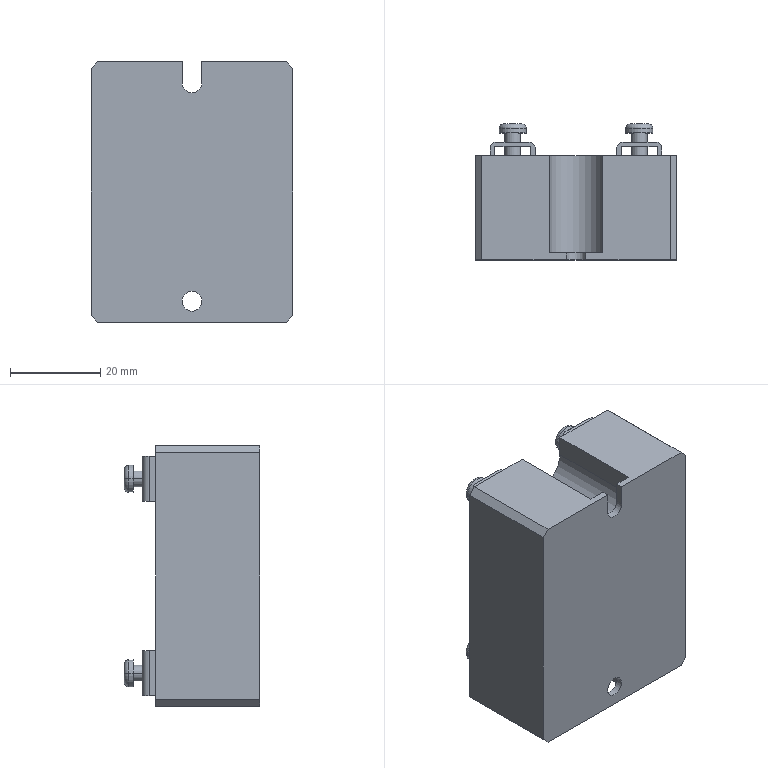Part | STEP file | Solid-state relay 1 | 1 solid | 109 faces | box 44.6 x 30 x 57.6 mm | volume 54499 mm3 | plane 64 | cylinder 37 | torus 8 | commonest cylinder face diameters 3.5 x16 3 x8 6 x8 4.4 x3 11.8 x2